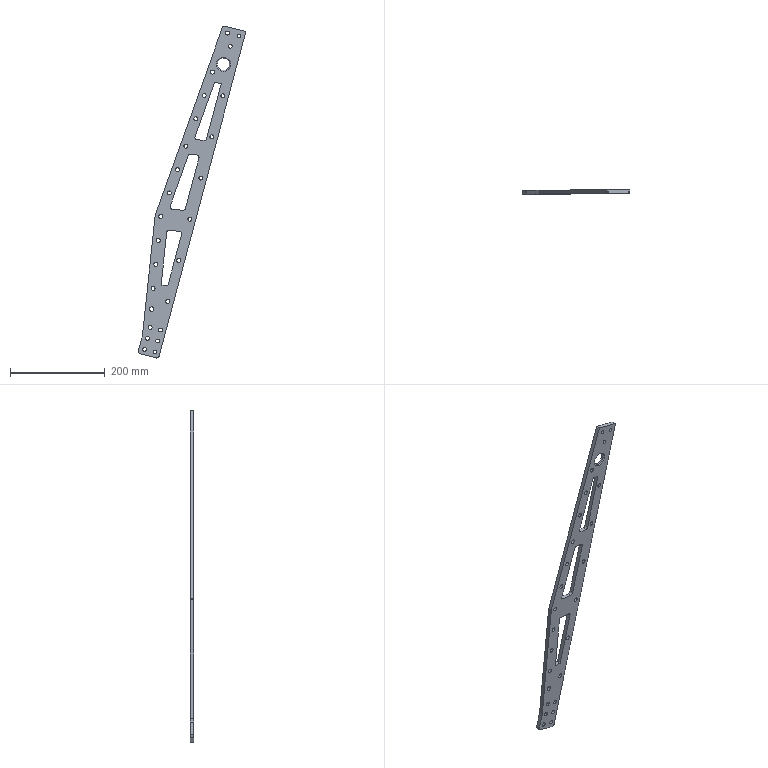Part | SolidWorks | features BaseBody 1 | 1 solid | 100 faces | box 226.999 x 8 x 701.792 mm | volume 290018 mm3 | cylinder 76 | plane 20 | cone 4 | commonest cylinder face diameters 8.4 x32 8.2 x18 10 x14 4 x5 6 x3 26 x2